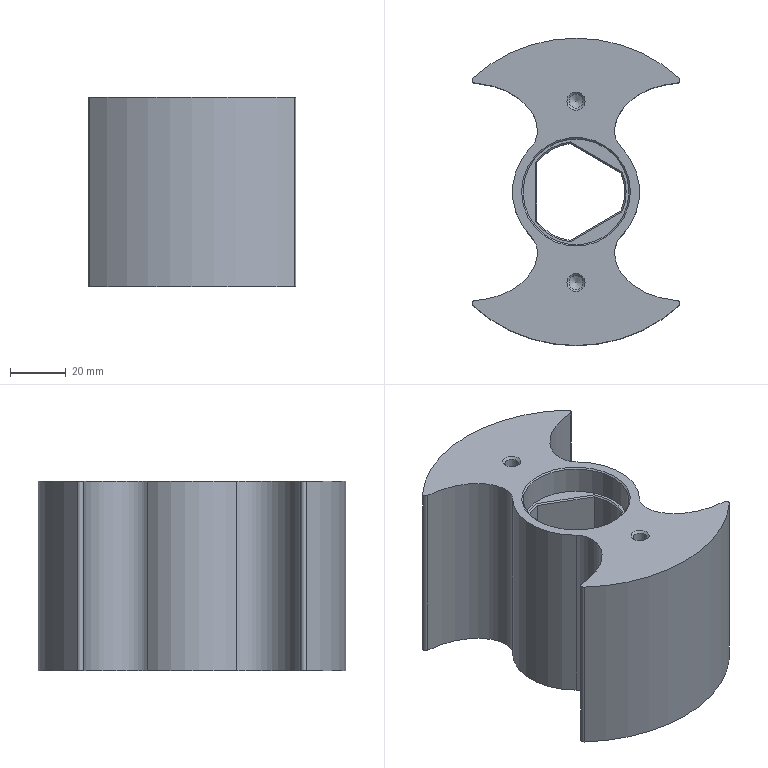NC program | NX | posted with a generic post | part box 74.46 x 110.159 x 68 mm
Lines 10216 to 11110 of 14265:
(刀补12 , TOOL : D12)
N20424 T12 M6
N20426 G54
N20428 G17 G0 G90 X-48.618 Y40.964 S5000 M3
N20430 G43 Z30. H12
N20432 Z1.
N20434 G94 G1 Z-1. F1250.
N20436 G41 X-48.525 Y40.926 D12
N20438 X-46.53 Y40.502
N20440 G3 X-45.388 Y40.873 R1.2
N20442 G2 X-32.988 Y36.627 R7.125
N20444 G3 X-31.64 Y29.822 R27.265
N20446 X-29.365 Y25.092 R20.862
N20448 X-26.715 Y22. R15.069
N20450 X-24.471 Y20.482 R10.273
N20452 X-22.513 Y19.857 R6.58
N20454 X-21.045 Y19.939 R3.496
N20456 X-20.344 Y20.344 R1.654
N20458 G2 X20.335 Y20.353 R28.771
N20460 G3 X21.045 Y19.939 R1.63
N20462 X22.513 Y19.857 R3.543
N20464 X24.572 Y20.533 R6.608
N20466 X27.243 Y22.489 R10.836
N20468 X29.871 Y25.911 R16.169
N20470 X31.8 Y30.311 R21.731
N20472 X32.988 Y36.632 R27.494
N20474 G2 X45.388 Y40.873 R7.125
N20476 G3 X46.53 Y40.502 R1.2
N20478 G1 X48.525 Y40.926
N20480 G40
N20482 X48.618 Y40.964
N20484 Z1.
N20486 G0 Z3.
N20488 X-48.618
N20490 Z0.
N20492 G1 Z-2.
N20494 G41 X-48.525 Y40.926
N20496 X-46.53 Y40.502
N20498 G3 X-45.388 Y40.873 R1.2
N20500 G2 X-32.988 Y36.627 R7.125
N20502 G3 X-31.64 Y29.822 R27.267
N20504 X-29.365 Y25.092 R20.86
N20506 X-26.715 Y22. R15.069
N20508 X-24.471 Y20.482 R10.274
N20510 X-22.513 Y19.857 R6.579
N20512 X-21.045 Y19.939 R3.496
N20514 X-20.344 Y20.344 R1.654
N20516 G2 X20.335 Y20.353 R28.771
N20518 G3 X21.045 Y19.939 R1.63
N20520 X22.513 Y19.857 R3.542
N20522 X24.572 Y20.533 R6.608
N20524 X27.243 Y22.489 R10.839
N20526 X29.871 Y25.911 R16.17
N20528 X31.8 Y30.311 R21.729
N20530 X32.988 Y36.632 R27.498
N20532 G2 X45.388 Y40.873 R7.125
N20534 G3 X46.53 Y40.502 R1.2
N20536 G1 X48.525 Y40.926
N20538 G40
N20540 X48.618 Y40.964
N20542 Z0.
N20544 G0 Z3.
N20546 X-48.618
N20548 Z-1.
N20550 G1 Z-3.
N20552 G41 X-48.525 Y40.926
N20554 X-46.53 Y40.502
N20556 G3 X-45.388 Y40.873 R1.2
N20558 G2 X-32.988 Y36.627 R7.125
N20560 G3 X-31.64 Y29.822 R27.268
N20562 X-29.365 Y25.092 R20.859
N20564 X-26.715 Y22. R15.068
N20566 X-24.471 Y20.482 R10.275
N20568 X-22.513 Y19.857 R6.578
N20570 X-21.045 Y19.939 R3.496
N20572 X-20.344 Y20.344 R1.655
N20574 G2 X20.335 Y20.353 R28.771
N20576 G3 X21.045 Y19.939 R1.63
N20578 X22.513 Y19.857 R3.542
N20580 X24.572 Y20.533 R6.608
N20582 X27.243 Y22.489 R10.841
N20584 X29.871 Y25.911 R16.171
N20586 X31.8 Y30.311 R21.727
N20588 X32.988 Y36.632 R27.502
N20590 G2 X45.388 Y40.873 R7.125
N20592 G3 X46.53 Y40.502 R1.2
N20594 G1 X48.525 Y40.926
N20596 G40
N20598 X48.618 Y40.964
N20600 Z-1.
N20602 G0 Z3.
N20604 X-48.618
N20606 Z-2.
N20608 G1 Z-4.
N20610 G41 X-48.525 Y40.926
N20612 X-46.53 Y40.502
N20614 G3 X-45.388 Y40.873 R1.2
N20616 G2 X-32.988 Y36.627 R7.125
N20618 G3 X-31.64 Y29.822 R27.27
N20620 X-29.365 Y25.092 R20.857
N20622 X-26.715 Y22. R15.068
N20624 X-24.471 Y20.482 R10.276
N20626 X-22.513 Y19.857 R6.578
N20628 X-21.045 Y19.939 R3.496
N20630 X-20.344 Y20.344 R1.655
N20632 G2 X20.335 Y20.353 R28.771
N20634 G3 X21.045 Y19.939 R1.631
N20636 X22.513 Y19.857 R3.542
N20638 X24.572 Y20.533 R6.608
N20640 X27.243 Y22.489 R10.829
N20642 X29.871 Y25.911 R16.172
N20644 X31.8 Y30.311 R21.727
N20646 X32.988 Y36.632 R27.543
N20648 G2 X45.388 Y40.873 R7.125
N20650 G3 X46.53 Y40.502 R1.2
N20652 G1 X48.525 Y40.926
N20654 G40
N20656 X48.618 Y40.964
N20658 Z-2.
N20660 G0 Z3.
N20662 X-48.618
N20664 Z-3.
N20666 G1 Z-5.
N20668 G41 X-48.525 Y40.926
N20670 X-46.53 Y40.502
N20672 G3 X-45.388 Y40.873 R1.2
N20674 G2 X-32.988 Y36.627 R7.125
N20676 G3 X-31.64 Y29.822 R27.272
N20678 X-29.365 Y25.092 R20.855
N20680 X-26.715 Y22. R15.068
N20682 X-24.471 Y20.482 R10.277
N20684 X-22.513 Y19.857 R6.577
N20686 X-21.045 Y19.939 R3.496
N20688 X-20.344 Y20.344 R1.655
N20690 G2 X20.335 Y20.353 R28.771
N20692 G3 X21.045 Y19.939 R1.631
N20694 X22.513 Y19.857 R3.541
N20696 X24.572 Y20.533 R6.608
N20698 X27.243 Y22.489 R10.831
N20700 X29.871 Y25.911 R16.173
N20702 X31.8 Y30.311 R21.727
N20704 X32.988 Y36.632 R27.543
N20706 G2 X45.388 Y40.873 R7.125
N20708 G3 X46.53 Y40.502 R1.2
N20710 G1 X48.525 Y40.926
N20712 G40
N20714 X48.618 Y40.964
N20716 Z-3.
N20718 G0 Z3.
N20720 X-48.618
N20722 Z-4.
N20724 G1 Z-6.
N20726 G41 X-48.525 Y40.926
N20728 X-46.53 Y40.502
N20730 G3 X-45.388 Y40.873 R1.2
N20732 G2 X-32.988 Y36.627 R7.125
N20734 G3 X-31.64 Y29.822 R27.273
N20736 X-29.365 Y25.092 R20.853
N20738 X-26.715 Y22. R15.068
N20740 X-24.471 Y20.482 R10.278
N20742 X-22.513 Y19.857 R6.576
N20744 X-21.045 Y19.939 R3.496
N20746 X-20.344 Y20.344 R1.656
N20748 G2 X20.335 Y20.353 R28.771
N20750 G3 X21.045 Y19.939 R1.631
N20752 X22.513 Y19.857 R3.541
N20754 X24.572 Y20.533 R6.608
N20756 X27.243 Y22.489 R10.833
N20758 X29.871 Y25.911 R16.149
N20760 X31.8 Y30.311 R21.728
N20762 X32.988 Y36.632 R27.544
N20764 G2 X45.388 Y40.873 R7.125
N20766 G3 X46.53 Y40.502 R1.2
N20768 G1 X48.525 Y40.926
N20770 G40
N20772 X48.618 Y40.964
N20774 Z-4.
N20776 G0 Z3.
N20778 X-48.618
N20780 Z-5.
N20782 G1 Z-7.
N20784 G41 X-48.525 Y40.926
N20786 X-46.53 Y40.502
N20788 G3 X-45.388 Y40.873 R1.2
N20790 G2 X-32.988 Y36.627 R7.125
N20792 G3 X-31.64 Y29.822 R27.275
N20794 X-29.365 Y25.092 R20.851
N20796 X-26.715 Y22. R15.068
N20798 X-24.471 Y20.482 R10.279
N20800 X-22.513 Y19.857 R6.575
N20802 X-21.045 Y19.94 R3.496
N20804 X-20.344 Y20.344 R1.656
N20806 G2 X20.335 Y20.353 R28.771
N20808 G3 X21.045 Y19.94 R1.632
N20810 X22.513 Y19.858 R3.541
N20812 X24.572 Y20.533 R6.608
N20814 X27.243 Y22.489 R10.835
N20816 X29.871 Y25.911 R16.15
N20818 X31.8 Y30.311 R21.728
N20820 X32.988 Y36.632 R27.544
N20822 G2 X45.388 Y40.873 R7.125
N20824 G3 X46.53 Y40.502 R1.2
N20826 G1 X48.525 Y40.926
N20828 G40
N20830 X48.618 Y40.964
N20832 Z-5.
N20834 G0 Z3.
N20836 X-48.618
N20838 Z-6.
N20840 G1 Z-8.
N20842 G41 X-48.525 Y40.926
N20844 X-46.53 Y40.502
N20846 G3 X-45.388 Y40.873 R1.2
N20848 G2 X-32.988 Y36.627 R7.125
N20850 G3 X-31.64 Y29.822 R27.277
N20852 X-29.365 Y25.092 R20.849
N20854 X-26.715 Y22. R15.068
N20856 X-24.471 Y20.482 R10.291
N20858 X-22.513 Y19.858 R6.575
N20860 X-21.045 Y19.94 R3.496
N20862 X-20.344 Y20.344 R1.656
N20864 G2 X20.335 Y20.353 R28.771
N20866 G3 X21.045 Y19.94 R1.632
N20868 X22.513 Y19.858 R3.54
N20870 X24.572 Y20.533 R6.608
N20872 X27.407 Y22.651 R10.999
N20874 X30.148 Y26.4 R16.769
N20876 X32.217 Y31.778 R22.996
N20878 X32.988 Y36.632 R28.224
N20880 G2 X45.388 Y40.873 R7.125
N20882 G3 X46.53 Y40.502 R1.2
N20884 G1 X48.525 Y40.926
N20886 G40
N20888 X48.618 Y40.964
N20890 Z-6.
N20892 G0 Z3.
N20894 X-48.618
N20896 Z-7.
N20898 G1 Z-9.
N20900 G41 X-48.525 Y40.926
N20902 X-46.53 Y40.502
N20904 G3 X-45.388 Y40.873 R1.2
N20906 G2 X-32.988 Y36.627 R7.125
N20908 G3 X-31.64 Y29.822 R27.278
N20910 X-29.365 Y25.092 R20.847
N20912 X-26.715 Y22. R15.068
N20914 X-24.471 Y20.482 R10.291
N20916 X-22.513 Y19.858 R6.574
N20918 X-21.045 Y19.94 R3.496
N20920 X-20.344 Y20.344 R1.657
N20922 G2 X20.335 Y20.353 R28.771
N20924 G3 X21.045 Y19.94 R1.632
N20926 X22.513 Y19.858 R3.54
N20928 X24.572 Y20.533 R6.608
N20930 X27.407 Y22.651 R11.001
N20932 X30.148 Y26.4 R16.768
N20934 X32.217 Y31.778 R22.995
N20936 X32.988 Y36.632 R28.232
N20938 G2 X45.388 Y40.873 R7.125
N20940 G3 X46.53 Y40.502 R1.2
N20942 G1 X48.525 Y40.926
N20944 G40
N20946 X48.618 Y40.964
N20948 Z-7.
N20950 G0 Z3.
N20952 X-48.618
N20954 Z-8.
N20956 G1 Z-10.
N20958 G41 X-48.525 Y40.926
N20960 X-46.53 Y40.502
N20962 G3 X-45.388 Y40.873 R1.2
N20964 G2 X-32.988 Y36.627 R7.125
N20966 G3 X-31.64 Y29.822 R27.28
N20968 X-29.365 Y25.092 R20.845
N20970 X-26.715 Y22. R15.068
N20972 X-24.471 Y20.482 R10.292
N20974 X-22.513 Y19.858 R6.573
N20976 X-21.045 Y19.94 R3.496
N20978 X-20.344 Y20.344 R1.657
N20980 G2 X20.335 Y20.353 R28.771
N20982 G3 X21.045 Y19.94 R1.633
N20984 X22.513 Y19.858 R3.539
N20986 X24.572 Y20.533 R6.608
N20988 X27.407 Y22.651 R11.004
N20990 X30.148 Y26.4 R16.766
N20992 X32.217 Y31.778 R22.995
N20994 X32.988 Y36.632 R28.239
N20996 G2 X45.388 Y40.873 R7.125
N20998 G3 X46.53 Y40.502 R1.2
N21000 G1 X48.525 Y40.926
N21002 G40
N21004 X48.618 Y40.964
N21006 Z-8.
N21008 G0 Z3.
N21010 X-48.618
N21012 Z-9.
N21014 G1 Z-11.
N21016 G41 X-48.525 Y40.926
N21018 X-46.53 Y40.502
N21020 G3 X-45.388 Y40.873 R1.2
N21022 G2 X-32.988 Y36.627 R7.125
N21024 G3 X-31.64 Y29.822 R27.282
N21026 X-29.365 Y25.092 R20.876
N21028 X-26.715 Y22. R15.068
N21030 X-24.471 Y20.482 R10.292
N21032 X-22.513 Y19.858 R6.572
N21034 X-21.045 Y19.94 R3.496
N21036 X-20.344 Y20.344 R1.657
N21038 G2 X20.335 Y20.353 R28.771
N21040 G3 X21.045 Y19.94 R1.633
N21042 X22.513 Y19.858 R3.539
N21044 X24.572 Y20.533 R6.608
N21046 X27.407 Y22.652 R11.006
N21048 X30.148 Y26.4 R16.765
N21050 X32.217 Y31.778 R23.021
N21052 X32.988 Y36.632 R28.247
N21054 G2 X45.388 Y40.873 R7.125
N21056 G3 X46.53 Y40.502 R1.2
N21058 G1 X48.525 Y40.926
N21060 G40
N21062 X48.618 Y40.964
N21064 Z-9.
N21066 G0 Z3.
N21068 X-48.618
N21070 Z-10.
N21072 G1 Z-12.
N21074 G41 X-48.525 Y40.926
N21076 X-46.53 Y40.502
N21078 G3 X-45.388 Y40.873 R1.2
N21080 G2 X-32.988 Y36.627 R7.125
N21082 G3 X-31.64 Y29.822 R27.283
N21084 X-29.365 Y25.092 R20.874
N21086 X-26.715 Y22. R15.068
N21088 X-24.471 Y20.482 R10.293
N21090 X-22.513 Y19.858 R6.572
N21092 X-21.045 Y19.94 R3.496
N21094 X-20.344 Y20.344 R1.658
N21096 G2 X20.335 Y20.353 R28.771
N21098 G3 X21.045 Y19.94 R1.633
N21100 X22.513 Y19.858 R3.539
N21102 X24.572 Y20.533 R6.608
N21104 X27.407 Y22.652 R11.009
N21106 X30.148 Y26.4 R16.764
N21108 X32.217 Y31.778 R23.018
N21110 X32.988 Y36.632 R28.255
N21112 G2 X45.388 Y40.873 R7.125
N21114 G3 X46.53 Y40.502 R1.2
N21116 G1 X48.525 Y40.926
N21118 G40
N21120 X48.618 Y40.964
N21122 Z-10.
N21124 G0 Z3.
N21126 X-48.618
N21128 Z-11.
N21130 G1 Z-13.
N21132 G41 X-48.525 Y40.926
N21134 X-46.53 Y40.502
N21136 G3 X-45.388 Y40.873 R1.2
N21138 G2 X-32.988 Y36.627 R7.125
N21140 G3 X-31.64 Y29.822 R27.285
N21142 X-29.365 Y25.092 R20.872
N21144 X-26.715 Y22. R15.068
N21146 X-24.471 Y20.482 R10.294
N21148 X-22.513 Y19.858 R6.571
N21150 X-21.045 Y19.94 R3.496
N21152 X-20.344 Y20.344 R1.658
N21154 G2 X20.335 Y20.353 R28.771
N21156 G3 X21.045 Y19.94 R1.634
N21158 X22.513 Y19.858 R3.538
N21160 X24.572 Y20.533 R6.608
N21162 X27.407 Y22.652 R11.012
N21164 X30.148 Y26.4 R16.763
N21166 X32.217 Y31.778 R23.015
N21168 X32.988 Y36.632 R28.262
N21170 G2 X45.388 Y40.873 R7.125
N21172 G3 X46.53 Y40.502 R1.2
N21174 G1 X48.525 Y40.926
N21176 G40
N21178 X48.618 Y40.964
N21180 Z-11.
N21182 G0 Z3.
N21184 X-48.618
N21186 Z-12.
N21188 G1 Z-14.
N21190 G41 X-48.525 Y40.926
N21192 X-46.53 Y40.502
N21194 G3 X-45.388 Y40.873 R1.2
N21196 G2 X-32.988 Y36.627 R7.125
N21198 G3 X-31.639 Y29.822 R27.287
N21200 X-29.365 Y25.092 R20.87
N21202 X-26.715 Y22. R15.068
N21204 X-24.471 Y20.482 R10.294
N21206 X-22.513 Y19.858 R6.57
N21208 X-21.045 Y19.94 R3.496
N21210 X-20.344 Y20.344 R1.658
N21212 G2 X20.335 Y20.353 R28.771
N21214 G3 X21.045 Y19.94 R1.634
N21216 X22.513 Y19.858 R3.538
N21218 X24.572 Y20.533 R6.608
N21220 X27.407 Y22.652 R11.014
N21222 X30.148 Y26.4 R16.762
N21224 X32.217 Y31.778 R23.012
N21226 X32.988 Y36.632 R28.27
N21228 G2 X45.388 Y40.873 R7.125
N21230 G3 X46.53 Y40.502 R1.2
N21232 G1 X48.525 Y40.926
N21234 G40
N21236 X48.618 Y40.964
N21238 Z-12.
N21240 G0 Z3.
N21242 X-48.618
N21244 Z-13.
N21246 G1 Z-15.
N21248 G41 X-48.525 Y40.926
N21250 X-46.53 Y40.502
N21252 G3 X-45.388 Y40.873 R1.2
N21254 G2 X-32.988 Y36.627 R7.125
N21256 G3 X-31.639 Y29.822 R27.288
N21258 X-29.365 Y25.093 R20.868
N21260 X-26.715 Y22. R15.068
N21262 X-24.471 Y20.482 R10.295
N21264 X-22.513 Y19.858 R6.57
N21266 X-21.045 Y19.94 R3.496
N21268 X-20.344 Y20.344 R1.659
N21270 G2 X20.335 Y20.353 R28.771
N21272 G3 X21.045 Y19.94 R1.634
N21274 X22.513 Y19.858 R3.538
N21276 X24.572 Y20.533 R6.608
N21278 X27.407 Y22.652 R11.017
N21280 X30.148 Y26.4 R16.76
N21282 X32.217 Y31.778 R23.009
N21284 X32.988 Y36.632 R28.278
N21286 G2 X45.388 Y40.873 R7.125
N21288 G3 X46.53 Y40.502 R1.2
N21290 G1 X48.525 Y40.926
N21292 G40
N21294 X48.618 Y40.964
N21296 Z-13.
N21298 G0 Z3.
N21300 X-48.618
N21302 Z-14.
N21304 G1 Z-16.
N21306 G41 X-48.525 Y40.926
N21308 X-46.53 Y40.502
N21310 G3 X-45.388 Y40.873 R1.2
N21312 G2 X-32.988 Y36.627 R7.125
N21314 G3 X-31.639 Y29.822 R27.29
N21316 X-29.365 Y25.093 R20.867
N21318 X-26.715 Y22. R15.068
N21320 X-24.471 Y20.482 R10.295
N21322 X-22.513 Y19.858 R6.569
N21324 X-21.045 Y19.94 R3.496
N21326 X-20.344 Y20.344 R1.659
N21328 G2 X20.335 Y20.353 R28.771
N21330 G3 X21.045 Y19.94 R1.635
N21332 X22.513 Y19.858 R3.537
N21334 X24.572 Y20.533 R6.608
N21336 X27.407 Y22.652 R11.02
N21338 X30.148 Y26.4 R16.783
N21340 X32.217 Y31.778 R23.006
N21342 X32.988 Y36.632 R28.285
N21344 G2 X45.388 Y40.873 R7.125
N21346 G3 X46.53 Y40.502 R1.2
N21348 G1 X48.525 Y40.926
N21350 G40
N21352 X48.618 Y40.964
N21354 Z-14.
N21356 G0 Z3.
N21358 X-48.618
N21360 Z-15.
N21362 G1 Z-17.
N21364 G41 X-48.525 Y40.926
N21366 X-46.53 Y40.502
N21368 G3 X-45.388 Y40.873 R1.2
N21370 G2 X-32.988 Y36.627 R7.125
N21372 G3 X-31.639 Y29.822 R27.292
N21374 X-29.365 Y25.093 R20.865
N21376 X-26.715 Y22. R15.068
N21378 X-24.471 Y20.482 R10.296
N21380 X-22.513 Y19.858 R6.568
N21382 X-21.045 Y19.94 R3.496
N21384 X-20.344 Y20.344 R1.659
N21386 G2 X20.335 Y20.353 R28.771
N21388 G3 X21.045 Y19.94 R1.635
N21390 X22.513 Y19.858 R3.537
N21392 X24.572 Y20.533 R6.608
N21394 X27.407 Y22.652 R11.022
N21396 X30.148 Y26.4 R16.782
N21398 X32.217 Y31.778 R23.003
N21400 X32.988 Y36.632 R28.293
N21402 G2 X45.388 Y40.873 R7.125
N21404 G3 X46.53 Y40.502 R1.2
N21406 G1 X48.525 Y40.926
N21408 G40
N21410 X48.618 Y40.964
N21412 Z-15.
N21414 G0 Z3.
N21416 X-48.618
N21418 Z-16.
N21420 G1 Z-18.
N21422 G41 X-48.525 Y40.926
N21424 X-46.53 Y40.502
N21426 G3 X-45.388 Y40.873 R1.2
N21428 G2 X-32.988 Y36.627 R7.125
N21430 G3 X-31.639 Y29.822 R27.294
N21432 X-29.365 Y25.093 R20.863
N21434 X-26.715 Y22. R15.068
N21436 X-24.471 Y20.482 R10.296
N21438 X-22.513 Y19.858 R6.567
N21440 X-21.045 Y19.94 R3.496
N21442 X-20.344 Y20.344 R1.66
N21444 G2 X20.335 Y20.353 R28.771
N21446 G3 X21.045 Y19.94 R1.635
N21448 X22.513 Y19.858 R3.536
N21450 X24.571 Y20.533 R6.608
N21452 X27.407 Y22.652 R11.025
N21454 X30.148 Y26.4 R16.781
N21456 X32.217 Y31.778 R23.
N21458 X32.988 Y36.632 R28.301
N21460 G2 X45.388 Y40.873 R7.125
N21462 G3 X46.53 Y40.502 R1.2
N21464 G1 X48.525 Y40.926
N21466 G40
N21468 X48.618 Y40.964
N21470 Z-16.
N21472 G0 Z3.
N21474 X-48.618
N21476 Z-17.
N21478 G1 Z-19.
N21480 G41 X-48.525 Y40.926
N21482 X-46.53 Y40.502
N21484 G3 X-45.388 Y40.873 R1.2
N21486 G2 X-32.988 Y36.627 R7.125
N21488 G3 X-31.639 Y29.822 R27.295
N21490 X-29.365 Y25.093 R20.861
N21492 X-26.715 Y22. R15.068
N21494 X-24.471 Y20.482 R10.297
N21496 X-22.513 Y19.858 R6.567
N21498 X-21.045 Y19.94 R3.495
N21500 X-20.344 Y20.344 R1.66
N21502 G2 X20.335 Y20.353 R28.771
N21504 G3 X21.045 Y19.94 R1.636
N21506 X22.513 Y19.858 R3.536
N21508 X24.571 Y20.533 R6.608
N21510 X27.407 Y22.652 R11.027
N21512 X30.148 Y26.4 R16.78
N21514 X32.217 Y31.778 R22.997
N21516 X32.988 Y36.632 R28.309
N21518 G2 X45.388 Y40.873 R7.125
N21520 G3 X46.53 Y40.502 R1.2
N21522 G1 X48.525 Y40.926
N21524 G40
N21526 X48.618 Y40.964
N21528 Z-17.
N21530 G0 Z3.
N21532 X-48.618
N21534 Z-18.
N21536 G1 Z-20.
N21538 G41 X-48.525 Y40.926
N21540 X-46.53 Y40.502
N21542 G3 X-45.388 Y40.873 R1.2
N21544 G2 X-32.988 Y36.627 R7.125
N21546 G3 X-31.639 Y29.822 R27.297
N21548 X-29.365 Y25.093 R20.859
N21550 X-26.715 Y22. R15.068
N21552 X-24.471 Y20.482 R10.298
N21554 X-22.513 Y19.858 R6.566
N21556 X-21.045 Y19.94 R3.495
N21558 X-20.344 Y20.344 R1.66
N21560 G2 X20.335 Y20.353 R28.771
N21562 G3 X21.045 Y19.94 R1.636
N21564 X22.513 Y19.858 R3.536
N21566 X24.571 Y20.533 R6.608
N21568 X27.407 Y22.652 R11.03
N21570 X30.148 Y26.4 R16.778
N21572 X32.217 Y31.778 R22.994
N21574 X32.988 Y36.632 R28.316
N21576 G2 X45.388 Y40.873 R7.125
N21578 G3 X46.53 Y40.502 R1.2
N21580 G1 X48.525 Y40.926
N21582 G40
N21584 X48.618 Y40.964
N21586 Z-18.
N21588 G0 Z3.
N21590 X-48.618
N21592 Z-19.
N21594 G1 Z-21.
N21596 G41 X-48.525 Y40.926
N21598 X-46.53 Y40.502
N21600 G3 X-45.388 Y40.873 R1.2
N21602 G2 X-32.988 Y36.627 R7.125
N21604 G3 X-31.639 Y29.822 R27.299
N21606 X-29.365 Y25.093 R20.857
N21608 X-26.715 Y22. R15.068
N21610 X-24.471 Y20.482 R10.298
N21612 X-22.513 Y19.858 R6.565
N21614 X-21.045 Y19.94 R3.495
N21616 X-20.344 Y20.344 R1.661
N21618 G2 X20.335 Y20.353 R28.771
N21620 G3 X21.045 Y19.94 R1.636
N21622 X22.513 Y19.858 R3.535
N21624 X24.571 Y20.533 R6.608
N21626 X27.407 Y22.652 R11.033
N21628 X30.148 Y26.4 R16.777
N21630 X32.216 Y31.778 R22.991
N21632 X32.988 Y36.632 R28.324
N21634 G2 X45.388 Y40.873 R7.125
N21636 G3 X46.53 Y40.502 R1.2
N21638 G1 X48.525 Y40.926
N21640 G40
N21642 X48.618 Y40.964
N21644 Z-19.
N21646 G0 Z3.
N21648 X-48.618
N21650 Z-20.
N21652 G1 Z-22.
N21654 G41 X-48.525 Y40.926
N21656 X-46.53 Y40.502
N21658 G3 X-45.388 Y40.873 R1.2
N21660 G2 X-32.988 Y36.627 R7.125
N21662 G3 X-31.639 Y29.822 R27.3
N21664 X-29.365 Y25.093 R20.855
N21666 X-26.715 Y22. R15.068
N21668 X-24.471 Y20.482 R10.299
N21670 X-22.513 Y19.858 R6.565
N21672 X-21.045 Y19.94 R3.495
N21674 X-20.344 Y20.344 R1.661
N21676 G2 X20.335 Y20.353 R28.771
N21678 G3 X21.045 Y19.94 R1.637
N21680 X22.513 Y19.858 R3.535
N21682 X24.571 Y20.533 R6.608
N21684 X27.407 Y22.652 R11.035
N21686 X30.148 Y26.4 R16.776
N21688 X32.216 Y31.778 R22.988
N21690 X32.988 Y36.632 R28.332
N21692 G2 X45.388 Y40.873 R7.125
N21694 G3 X46.53 Y40.502 R1.2
N21696 G1 X48.525 Y40.926
N21698 G40
N21700 X48.618 Y40.964
N21702 Z-20.
N21704 G0 Z3.
N21706 X-48.618
N21708 Z-21.
N21710 G1 Z-23.
N21712 G41 X-48.525 Y40.926
N21714 X-46.53 Y40.502
N21716 G3 X-45.388 Y40.873 R1.2
N21718 G2 X-32.988 Y36.627 R7.125
N21720 G3 X-31.639 Y29.822 R27.302
N21722 X-29.365 Y25.093 R20.853
N21724 X-26.715 Y22. R15.068
N21726 X-24.471 Y20.482 R10.299
N21728 X-22.513 Y19.858 R6.564
N21730 X-21.045 Y19.94 R3.495
N21732 X-20.344 Y20.344 R1.661
N21734 G2 X20.335 Y20.353 R28.771
N21736 G3 X21.045 Y19.94 R1.637
N21738 X22.513 Y19.858 R3.535
N21740 X24.571 Y20.533 R6.608
N21742 X27.407 Y22.652 R11.038
N21744 X30.148 Y26.4 R16.775
N21746 X32.216 Y31.778 R22.985
N21748 X32.988 Y36.632 R28.339
N21750 G2 X45.388 Y40.873 R7.125
N21752 G3 X46.53 Y40.502 R1.2
N21754 G1 X48.525 Y40.926
N21756 G40
N21758 X48.618 Y40.964
N21760 Z-21.
N21762 G0 Z3.
N21764 X-48.618
N21766 Z-22.
N21768 G1 Z-24.
N21770 G41 X-48.525 Y40.926
N21772 X-46.53 Y40.502
N21774 G3 X-45.388 Y40.873 R1.2
N21776 G2 X-32.988 Y36.627 R7.125
N21778 G3 X-31.639 Y29.822 R27.324
N21780 X-29.365 Y25.093 R20.851
N21782 X-26.715 Y22. R15.068
N21784 X-24.471 Y20.483 R10.3
N21786 X-22.513 Y19.858 R6.563
N21788 X-21.045 Y19.94 R3.495
N21790 X-20.344 Y20.344 R1.662
N21792 G2 X20.335 Y20.353 R28.771
N21794 G3 X21.045 Y19.94 R1.637
N21796 X22.513 Y19.858 R3.534
N21798 X24.571 Y20.533 R6.608
N21800 X27.407 Y22.652 R11.041
N21802 X30.148 Y26.4 R16.774
N21804 X32.216 Y31.778 R22.982
N21806 X32.988 Y36.632 R28.347
N21808 G2 X45.388 Y40.873 R7.125
N21810 G3 X46.53 Y40.502 R1.2
N21812 G1 X48.525 Y40.926
N21814 G40
N21816 X48.618 Y40.964
N21818 Z-22.
N21820 G0 Z3.
N21822 X-48.618
N21824 Z-23.
N21826 G1 Z-25.
N21828 G41 X-48.525 Y40.926
N21830 X-46.53 Y40.502
N21832 G3 X-45.388 Y40.873 R1.2
N21834 G2 X-32.988 Y36.627 R7.125
N21836 G3 X-31.639 Y29.822 R27.324
N21838 X-29.365 Y25.093 R20.849
N21840 X-26.715 Y22. R15.068
N21842 X-24.471 Y20.483 R10.3
N21844 X-22.513 Y19.858 R6.562
N21846 X-21.045 Y19.94 R3.495
N21848 X-20.344 Y20.344 R1.662
N21850 G2 X20.335 Y20.353 R28.771
N21852 G3 X21.045 Y19.94 R1.638
N21854 X22.513 Y19.858 R3.534
N21856 X24.571 Y20.533 R6.608
N21858 X27.407 Y22.652 R11.043
N21860 X30.148 Y26.4 R16.773
N21862 X32.216 Y31.778 R22.979
N21864 X32.988 Y36.632 R28.355
N21866 G2 X45.388 Y40.873 R7.125
N21868 G3 X46.53 Y40.502 R1.2
N21870 G1 X48.525 Y40.926
N21872 G40
N21874 X48.618 Y40.964
N21876 Z-23.
N21878 G0 Z3.
N21880 X-48.618
N21882 Z-24.
N21884 G1 Z-26.
N21886 G41 X-48.525 Y40.926
N21888 X-46.53 Y40.502
N21890 G3 X-45.388 Y40.873 R1.2
N21892 G2 X-32.988 Y36.627 R7.125
N21894 G3 X-31.639 Y29.822 R27.325
N21896 X-29.365 Y25.093 R20.848
N21898 X-26.714 Y22. R15.068
N21900 X-24.471 Y20.483 R10.301
N21902 X-22.513 Y19.858 R6.562
N21904 X-21.045 Y19.94 R3.495
N21906 X-20.344 Y20.344 R1.662
N21908 G2 X20.335 Y20.353 R28.771
N21910 G3 X21.045 Y19.94 R1.638
N21912 X22.513 Y19.858 R3.533
N21914 X24.571 Y20.533 R6.608
N21916 X27.407 Y22.652 R11.046
N21918 X30.148 Y26.4 R16.771
N21920 X32.216 Y31.778 R22.975
N21922 X32.988 Y36.632 R28.363
N21924 G2 X45.388 Y40.873 R7.125
N21926 G3 X46.53 Y40.502 R1.2
N21928 G1 X48.525 Y40.926
N21930 G40
N21932 X48.618 Y40.964
N21934 Z-24.
N21936 G0 Z3.
N21938 X-48.618
N21940 Z-25.
N21942 G1 Z-27.
N21944 G41 X-48.525 Y40.926
N21946 X-46.53 Y40.502
N21948 G3 X-45.388 Y40.873 R1.2
N21950 G2 X-32.988 Y36.627 R7.125
N21952 G3 X-31.639 Y29.822 R27.325
N21954 X-29.365 Y25.093 R20.846
N21956 X-26.714 Y22. R15.068
N21958 X-24.471 Y20.483 R10.301
N21960 X-22.513 Y19.858 R6.561
N21962 X-21.045 Y19.94 R3.495
N21964 X-20.344 Y20.344 R1.663
N21966 G2 X20.335 Y20.353 R28.771
N21968 G3 X21.045 Y19.94 R1.638
N21970 X22.513 Y19.858 R3.533
N21972 X24.571 Y20.533 R6.608
N21974 X27.407 Y22.652 R11.048
N21976 X30.148 Y26.4 R16.77
N21978 X32.216 Y31.778 R22.972
N21980 X32.988 Y36.632 R28.37
N21982 G2 X45.388 Y40.873 R7.125
N21984 G3 X46.53 Y40.502 R1.2
N21986 G1 X48.525 Y40.926
N21988 G40
N21990 X48.618 Y40.964
N21992 Z-25.
N21994 G0 Z3.
N21996 X-48.618
N21998 Z-26.
N22000 G1 Z-28.
N22002 G41 X-48.525 Y40.926
N22004 X-46.53 Y40.502
N22006 G3 X-45.388 Y40.873 R1.2
N22008 G2 X-32.988 Y36.627 R7.125
N22010 G3 X-31.639 Y29.822 R27.325
N22012 X-29.365 Y25.093 R20.844
N22014 X-26.714 Y22. R15.068
N22016 X-24.471 Y20.483 R10.302
N22018 X-22.513 Y19.858 R6.56
N22020 X-21.045 Y19.94 R3.495
N22022 X-20.344 Y20.344 R1.663
N22024 G2 X20.335 Y20.353 R28.771
N22026 G3 X21.045 Y19.94 R1.639
N22028 X22.513 Y19.859 R3.533
N22030 X24.571 Y20.533 R6.608
N22032 X27.407 Y22.652 R11.051
N22034 X30.147 Y26.4 R16.769
N22036 X32.216 Y31.778 R22.969
N22038 X32.988 Y36.632 R28.378
N22040 G2 X45.388 Y40.873 R7.125
N22042 G3 X46.53 Y40.502 R1.2
N22044 G1 X48.525 Y40.926
N22046 G40
N22048 X48.618 Y40.964
N22050 Z-26.
N22052 G0 Z3.
N22054 X-48.618
N22056 Z-27.
N22058 G1 Z-29.
N22060 G41 X-48.525 Y40.926
N22062 X-46.53 Y40.502
N22064 G3 X-45.388 Y40.873 R1.2
N22066 G2 X-32.988 Y36.627 R7.125
N22068 G3 X-31.639 Y29.822 R27.326
N22070 X-29.365 Y25.093 R20.842
N22072 X-26.714 Y22. R15.086
N22074 X-24.471 Y20.483 R10.303
N22076 X-22.513 Y19.858 R6.56
N22078 X-21.045 Y19.94 R3.495
N22080 X-20.344 Y20.344 R1.663
N22082 G2 X20.335 Y20.353 R28.771
N22084 G3 X21.045 Y19.94 R1.639
N22086 X22.513 Y19.859 R3.532
N22088 X24.571 Y20.533 R6.608
N22090 X27.407 Y22.652 R11.054
N22092 X30.147 Y26.4 R16.768
N22094 X32.216 Y31.778 R22.966
N22096 X32.988 Y36.632 R28.384
N22098 G2 X45.388 Y40.873 R7.125
N22100 G3 X46.53 Y40.502 R1.2
N22102 G1 X48.525 Y40.926
N22104 G40
N22106 X48.618 Y40.964
N22108 Z-27.
N22110 G0 Z3.
N22112 X-48.618
N22114 Z-28.
N22116 G1 Z-30.
N22118 G41 X-48.525 Y40.926
N22120 X-46.53 Y40.502
N22122 G3 X-45.388 Y40.873 R1.2
N22124 G2 X-32.988 Y36.627 R7.125
N22126 G3 X-31.639 Y29.822 R27.326
N22128 X-29.365 Y25.093 R20.84
N22130 X-26.714 Y22. R15.085
N22132 X-24.471 Y20.483 R10.303
N22134 X-22.513 Y19.858 R6.559
N22136 X-21.045 Y19.94 R3.495
N22138 X-20.344 Y20.344 R1.664
N22140 G2 X20.335 Y20.353 R28.771
N22142 G3 X21.045 Y19.94 R1.639
N22144 X22.513 Y19.859 R3.532
N22146 X24.571 Y20.533 R6.608
N22148 X27.407 Y22.652 R11.056
N22150 X30.147 Y26.4 R16.767
N22152 X32.216 Y31.778 R22.963
N22154 X32.988 Y36.632 R28.387
N22156 G2 X45.388 Y40.873 R7.125
N22158 G3 X46.53 Y40.502 R1.2
N22160 G1 X48.525 Y40.926
N22162 G40
N22164 X48.618 Y40.964
N22166 Z-28.
N22168 G0 Z3.
N22170 X-48.618
N22172 Z-29.
N22174 G1 Z-31.
N22176 G41 X-48.525 Y40.926
N22178 X-46.53 Y40.502
N22180 G3 X-45.388 Y40.873 R1.2
N22182 G2 X-32.988 Y36.627 R7.125
N22184 G3 X-31.639 Y29.822 R27.327
N22186 X-29.365 Y25.093 R20.85
N22188 X-26.714 Y22. R15.084
N22190 X-24.471 Y20.483 R10.304
N22192 X-22.513 Y19.859 R6.558
N22194 X-21.045 Y19.94 R3.495
N22196 X-20.344 Y20.344 R1.664
N22198 G2 X20.335 Y20.353 R28.771
N22200 G3 X21.045 Y19.94 R1.64
N22202 X22.513 Y19.859 R3.532
N22204 X24.571 Y20.533 R6.608
N22206 X27.407 Y22.652 R11.057